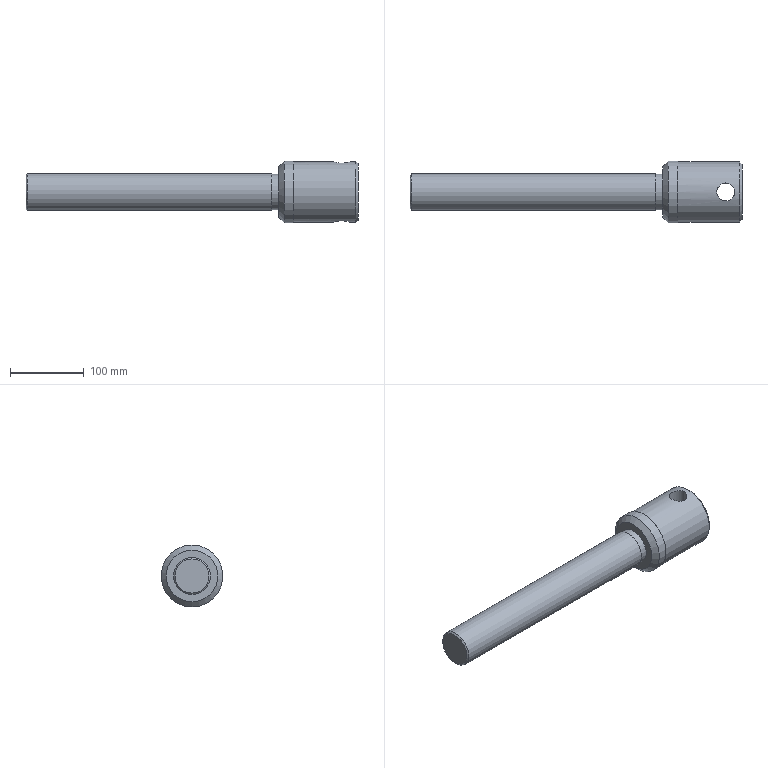Part | NX | features 侧推千斤顶活塞 2 | 1 solid | 13 faces | box 449.94 x 84 x 84 mm | volume 1201706 mm3 | plane 5 | cylinder 5 | cone 3 | commonest cylinder face diameters 24.29 x1 48 x1 50.16 x1 82 x1 84 x1
STEP:
#1=CARTESIAN_POINT('',(0.,0.,23.08));
#2=VERTEX_POINT('',#1);
#3=CARTESIAN_POINT('',(0.,0.,0.));
#4=DIRECTION('',(-1.,0.,0.));
#5=DIRECTION('',(0.,0.,1.));
#6=AXIS2_PLACEMENT_3D('',#3,#4,#5);
#7=CIRCLE('',#6,23.08);
#8=EDGE_CURVE('',#2,#2,#7,.T.);
#9=ORIENTED_EDGE('',*,*,#8,.T.);
#10=EDGE_LOOP('',(#9));
#11=FACE_BOUND('',#10,.T.);
#12=CARTESIAN_POINT('',(0.,0.,0.));
#13=DIRECTION('',(1.,0.,0.));
#14=DIRECTION('',(0.,0.,-1.));
#15=AXIS2_PLACEMENT_3D('',#12,#13,#14);
#16=PLANE('',#15);
#17=ADVANCED_FACE('',(#11),#16,.F.);
#18=ORIENTED_EDGE('',*,*,#8,.F.);
#19=EDGE_LOOP('',(#18));
#20=FACE_BOUND('',#19,.T.);
#21=CARTESIAN_POINT('',(2.,0.,25.08));
#22=VERTEX_POINT('',#21);
#23=CARTESIAN_POINT('',(2.,0.,0.));
#24=DIRECTION('',(-1.,0.,0.));
#25=DIRECTION('',(0.,0.,1.));
#26=AXIS2_PLACEMENT_3D('',#23,#24,#25);
#27=CIRCLE('',#26,25.08);
#28=EDGE_CURVE('',#22,#22,#27,.T.);
#29=ORIENTED_EDGE('',*,*,#28,.T.);
#30=EDGE_LOOP('',(#29));
#31=FACE_BOUND('',#30,.T.);
#32=CARTESIAN_POINT('',(2.,0.,0.));
#33=DIRECTION('',(1.,0.,0.));
#34=DIRECTION('',(0.,0.,-1.));
#35=AXIS2_PLACEMENT_3D('',#32,#33,#34);
#36=CONICAL_SURFACE('',#35,25.08,0.7854);
#37=ADVANCED_FACE('',(#20,#31),#36,.T.);
#38=ORIENTED_EDGE('',*,*,#28,.F.);
#39=EDGE_LOOP('',(#38));
#40=FACE_BOUND('',#39,.T.);
#41=CARTESIAN_POINT('',(332.85,0.,25.08));
#42=VERTEX_POINT('',#41);
#43=CARTESIAN_POINT('',(332.85,0.,0.));
#44=DIRECTION('',(-1.,0.,0.));
#45=DIRECTION('',(0.,0.,1.));
#46=AXIS2_PLACEMENT_3D('',#43,#44,#45);
#47=CIRCLE('',#46,25.08);
#48=EDGE_CURVE('',#42,#42,#47,.T.);
#49=ORIENTED_EDGE('',*,*,#48,.T.);
#50=EDGE_LOOP('',(#49));
#51=FACE_BOUND('',#50,.T.);
#52=CARTESIAN_POINT('',(0.,0.,0.));
#53=DIRECTION('',(-1.,0.,0.));
#54=DIRECTION('',(0.,0.,1.));
#55=AXIS2_PLACEMENT_3D('',#52,#53,#54);
#56=CYLINDRICAL_SURFACE('',#55,25.08);
#57=ADVANCED_FACE('',(#40,#51),#56,.T.);
#58=ORIENTED_EDGE('',*,*,#48,.F.);
#59=EDGE_LOOP('',(#58));
#60=FACE_BOUND('',#59,.T.);
#61=CARTESIAN_POINT('',(332.85,0.,24.));
#62=VERTEX_POINT('',#61);
#63=CARTESIAN_POINT('',(332.85,0.,0.));
#64=DIRECTION('',(-1.,0.,0.));
#65=DIRECTION('',(0.,0.,1.));
#66=AXIS2_PLACEMENT_3D('',#63,#64,#65);
#67=CIRCLE('',#66,24.);
#68=EDGE_CURVE('',#62,#62,#67,.T.);
#69=ORIENTED_EDGE('',*,*,#68,.T.);
#70=EDGE_LOOP('',(#69));
#71=FACE_BOUND('',#70,.T.);
#72=CARTESIAN_POINT('',(332.85,25.08,0.));
#73=DIRECTION('',(-1.,0.,0.));
#74=DIRECTION('',(0.,0.,1.));
#75=AXIS2_PLACEMENT_3D('',#72,#73,#74);
#76=PLANE('',#75);
#77=ADVANCED_FACE('',(#60,#71),#76,.F.);
#78=ORIENTED_EDGE('',*,*,#68,.F.);
#79=EDGE_LOOP('',(#78));
#80=FACE_BOUND('',#79,.T.);
#81=CARTESIAN_POINT('',(342.73,0.,24.));
#82=VERTEX_POINT('',#81);
#83=CARTESIAN_POINT('',(342.73,0.,0.));
#84=DIRECTION('',(-1.,0.,0.));
#85=DIRECTION('',(0.,0.,1.));
#86=AXIS2_PLACEMENT_3D('',#83,#84,#85);
#87=CIRCLE('',#86,24.);
#88=EDGE_CURVE('',#82,#82,#87,.T.);
#89=ORIENTED_EDGE('',*,*,#88,.T.);
#90=EDGE_LOOP('',(#89));
#91=FACE_BOUND('',#90,.T.);
#92=CARTESIAN_POINT('',(0.,0.,0.));
#93=DIRECTION('',(-1.,0.,0.));
#94=DIRECTION('',(0.,0.,1.));
#95=AXIS2_PLACEMENT_3D('',#92,#93,#94);
#96=CYLINDRICAL_SURFACE('',#95,24.);
#97=ADVANCED_FACE('',(#80,#91),#96,.T.);
#98=ORIENTED_EDGE('',*,*,#88,.F.);
#99=EDGE_LOOP('',(#98));
#100=FACE_BOUND('',#99,.T.);
#101=CARTESIAN_POINT('',(342.73,0.,34.86));
#102=VERTEX_POINT('',#101);
#103=CARTESIAN_POINT('',(342.73,0.,0.));
#104=DIRECTION('',(-1.,0.,0.));
#105=DIRECTION('',(0.,0.,1.));
#106=AXIS2_PLACEMENT_3D('',#103,#104,#105);
#107=CIRCLE('',#106,34.86);
#108=EDGE_CURVE('',#102,#102,#107,.T.);
#109=ORIENTED_EDGE('',*,*,#108,.T.);
#110=EDGE_LOOP('',(#109));
#111=FACE_BOUND('',#110,.T.);
#112=CARTESIAN_POINT('',(342.73,24.,0.));
#113=DIRECTION('',(1.,0.,0.));
#114=DIRECTION('',(0.,0.,-1.));
#115=AXIS2_PLACEMENT_3D('',#112,#113,#114);
#116=PLANE('',#115);
#117=ADVANCED_FACE('',(#100,#111),#116,.F.);
#118=ORIENTED_EDGE('',*,*,#108,.F.);
#119=EDGE_LOOP('',(#118));
#120=FACE_BOUND('',#119,.T.);
#121=CARTESIAN_POINT('',(349.87,0.,42.));
#122=VERTEX_POINT('',#121);
#123=CARTESIAN_POINT('',(349.87,0.,0.));
#124=DIRECTION('',(-1.,0.,0.));
#125=DIRECTION('',(0.,0.,1.));
#126=AXIS2_PLACEMENT_3D('',#123,#124,#125);
#127=CIRCLE('',#126,42.);
#128=EDGE_CURVE('',#122,#122,#127,.T.);
#129=ORIENTED_EDGE('',*,*,#128,.T.);
#130=EDGE_LOOP('',(#129));
#131=FACE_BOUND('',#130,.T.);
#132=CARTESIAN_POINT('',(349.87,0.,0.));
#133=DIRECTION('',(1.,0.,0.));
#134=DIRECTION('',(0.,0.,-1.));
#135=AXIS2_PLACEMENT_3D('',#132,#133,#134);
#136=CONICAL_SURFACE('',#135,42.,0.7854);
#137=ADVANCED_FACE('',(#120,#131),#136,.T.);
#138=ORIENTED_EDGE('',*,*,#128,.F.);
#139=EDGE_LOOP('',(#138));
#140=FACE_BOUND('',#139,.T.);
#141=CARTESIAN_POINT('',(362.94,0.,42.));
#142=VERTEX_POINT('',#141);
#143=CARTESIAN_POINT('',(362.94,0.,0.));
#144=DIRECTION('',(-1.,0.,0.));
#145=DIRECTION('',(0.,0.,1.));
#146=AXIS2_PLACEMENT_3D('',#143,#144,#145);
#147=CIRCLE('',#146,42.);
#148=EDGE_CURVE('',#142,#142,#147,.T.);
#149=ORIENTED_EDGE('',*,*,#148,.T.);
#150=EDGE_LOOP('',(#149));
#151=FACE_BOUND('',#150,.T.);
#152=CARTESIAN_POINT('',(0.,0.,0.));
#153=DIRECTION('',(-1.,0.,0.));
#154=DIRECTION('',(0.,0.,1.));
#155=AXIS2_PLACEMENT_3D('',#152,#153,#154);
#156=CYLINDRICAL_SURFACE('',#155,42.);
#157=ADVANCED_FACE('',(#140,#151),#156,.T.);
#158=ORIENTED_EDGE('',*,*,#148,.F.);
#159=EDGE_LOOP('',(#158));
#160=FACE_BOUND('',#159,.T.);
#161=CARTESIAN_POINT('',(362.94,0.,41.));
#162=VERTEX_POINT('',#161);
#163=CARTESIAN_POINT('',(362.94,0.,0.));
#164=DIRECTION('',(-1.,0.,0.));
#165=DIRECTION('',(0.,0.,1.));
#166=AXIS2_PLACEMENT_3D('',#163,#164,#165);
#167=CIRCLE('',#166,41.);
#168=EDGE_CURVE('',#162,#162,#167,.T.);
#169=ORIENTED_EDGE('',*,*,#168,.T.);
#170=EDGE_LOOP('',(#169));
#171=FACE_BOUND('',#170,.T.);
#172=CARTESIAN_POINT('',(362.94,42.,0.));
#173=DIRECTION('',(-1.,0.,0.));
#174=DIRECTION('',(0.,0.,1.));
#175=AXIS2_PLACEMENT_3D('',#172,#173,#174);
#176=PLANE('',#175);
#177=ADVANCED_FACE('',(#160,#171),#176,.F.);
#178=CARTESIAN_POINT('',(440.085,0.,41.));
#179=VERTEX_POINT('',#178);
#180=CARTESIAN_POINT('',(439.438,4.806,40.802));
#181=CARTESIAN_POINT('',(440.408,-0.002211,41.099));
#182=CARTESIAN_POINT('',(439.441,-4.797,40.802));
#183=CARTESIAN_POINT('',(436.744,-8.811,40.092));
#184=CARTESIAN_POINT('',(432.735,-11.5,39.368));
#185=CARTESIAN_POINT('',(427.95,-12.466,39.056));
#186=CARTESIAN_POINT('',(423.153,-11.506,39.366));
#187=CARTESIAN_POINT('',(419.13,-8.807,40.093));
#188=CARTESIAN_POINT('',(416.438,-4.793,40.803));
#189=CARTESIAN_POINT('',(415.474,-0.005926,41.098));
#190=CARTESIAN_POINT('',(416.434,4.785,40.804));
#191=CARTESIAN_POINT('',(419.128,8.804,40.094));
#192=CARTESIAN_POINT('',(423.143,11.501,39.368));
#193=CARTESIAN_POINT('',(427.936,12.466,39.056));
#194=CARTESIAN_POINT('',(432.729,11.504,39.367));
#195=CARTESIAN_POINT('',(436.743,8.811,40.092));
#196=CARTESIAN_POINT('',(439.438,4.806,40.802));
#197=CARTESIAN_POINT('',(440.408,-0.002211,41.099));
#198=CARTESIAN_POINT('',(439.441,-4.797,40.802));
#199=B_SPLINE_CURVE_WITH_KNOTS('',3,(#180,#181,#182,#183,#184,#185,#186,#187,#188,#189,#190,#191,#192,#193,#194,#195,#196,#197,#198),.UNSPECIFIED.,.T.,.F.,(1,1,1,1,1,1,1,1,1,1,1,1,1,1,1,1,1,1,1,1,1,1,1),(-0.01432,-0.009545,-0.004773,0.,0.004773,0.009545,0.01432,0.01909,0.02386,0.02864,0.03341,0.03818,0.04295,0.04773,0.0525,0.05727,0.06204,0.06682,0.07159,0.07636,0.08113,0.08591,0.09068),.UNSPECIFIED.);
#200=EDGE_CURVE('',#179,#179,#199,.T.);
#201=ORIENTED_EDGE('',*,*,#200,.T.);
#202=EDGE_LOOP('',(#201));
#203=FACE_BOUND('',#202,.T.);
#204=CARTESIAN_POINT('',(440.085,0.,-41.));
#205=VERTEX_POINT('',#204);
#206=CARTESIAN_POINT('',(439.438,-4.806,-40.802));
#207=CARTESIAN_POINT('',(440.408,0.002211,-41.099));
#208=CARTESIAN_POINT('',(439.441,4.797,-40.802));
#209=CARTESIAN_POINT('',(436.744,8.811,-40.092));
#210=CARTESIAN_POINT('',(432.735,11.5,-39.368));
#211=CARTESIAN_POINT('',(427.95,12.466,-39.056));
#212=CARTESIAN_POINT('',(423.153,11.506,-39.366));
#213=CARTESIAN_POINT('',(419.13,8.807,-40.093));
#214=CARTESIAN_POINT('',(416.438,4.793,-40.803));
#215=CARTESIAN_POINT('',(415.474,0.005926,-41.098));
#216=CARTESIAN_POINT('',(416.434,-4.785,-40.804));
#217=CARTESIAN_POINT('',(419.128,-8.804,-40.094));
#218=CARTESIAN_POINT('',(423.143,-11.501,-39.368));
#219=CARTESIAN_POINT('',(427.936,-12.466,-39.056));
#220=CARTESIAN_POINT('',(432.729,-11.504,-39.367));
#221=CARTESIAN_POINT('',(436.743,-8.811,-40.092));
#222=CARTESIAN_POINT('',(439.438,-4.806,-40.802));
#223=CARTESIAN_POINT('',(440.408,0.002211,-41.099));
#224=CARTESIAN_POINT('',(439.441,4.797,-40.802));
#225=B_SPLINE_CURVE_WITH_KNOTS('',3,(#206,#207,#208,#209,#210,#211,#212,#213,#214,#215,#216,#217,#218,#219,#220,#221,#222,#223,#224),.UNSPECIFIED.,.T.,.F.,(1,1,1,1,1,1,1,1,1,1,1,1,1,1,1,1,1,1,1,1,1,1,1),(-0.01432,-0.009545,-0.004773,0.,0.004773,0.009545,0.01432,0.01909,0.02386,0.02864,0.03341,0.03818,0.04295,0.04773,0.0525,0.05727,0.06204,0.06682,0.07159,0.07636,0.08113,0.08591,0.09068),.UNSPECIFIED.);
#226=EDGE_CURVE('',#205,#205,#225,.T.);
#227=ORIENTED_EDGE('',*,*,#226,.T.);
#228=EDGE_LOOP('',(#227));
#229=FACE_BOUND('',#228,.T.);
#230=ORIENTED_EDGE('',*,*,#168,.F.);
#231=EDGE_LOOP('',(#230));
#232=FACE_BOUND('',#231,.T.);
#233=CARTESIAN_POINT('',(446.94,0.,41.));
#234=VERTEX_POINT('',#233);
#235=CARTESIAN_POINT('',(446.94,0.,0.));
#236=DIRECTION('',(-1.,0.,0.));
#237=DIRECTION('',(0.,0.,1.));
#238=AXIS2_PLACEMENT_3D('',#235,#236,#237);
#239=CIRCLE('',#238,41.);
#240=EDGE_CURVE('',#234,#234,#239,.T.);
#241=ORIENTED_EDGE('',*,*,#240,.T.);
#242=EDGE_LOOP('',(#241));
#243=FACE_BOUND('',#242,.T.);
#244=CARTESIAN_POINT('',(0.,0.,0.));
#245=DIRECTION('',(-1.,0.,0.));
#246=DIRECTION('',(0.,0.,1.));
#247=AXIS2_PLACEMENT_3D('',#244,#245,#246);
#248=CYLINDRICAL_SURFACE('',#247,41.);
#249=ADVANCED_FACE('',(#203,#229,#232,#243),#248,.T.);
#250=ORIENTED_EDGE('',*,*,#240,.F.);
#251=EDGE_LOOP('',(#250));
#252=FACE_BOUND('',#251,.T.);
#253=CARTESIAN_POINT('',(449.94,0.,38.));
#254=VERTEX_POINT('',#253);
#255=CARTESIAN_POINT('',(449.94,0.,0.));
#256=DIRECTION('',(-1.,0.,0.));
#257=DIRECTION('',(0.,0.,1.));
#258=AXIS2_PLACEMENT_3D('',#255,#256,#257);
#259=CIRCLE('',#258,38.);
#260=EDGE_CURVE('',#254,#254,#259,.T.);
#261=ORIENTED_EDGE('',*,*,#260,.T.);
#262=EDGE_LOOP('',(#261));
#263=FACE_BOUND('',#262,.T.);
#264=CARTESIAN_POINT('',(449.94,0.,0.));
#265=DIRECTION('',(-1.,0.,0.));
#266=DIRECTION('',(0.,0.,1.));
#267=AXIS2_PLACEMENT_3D('',#264,#265,#266);
#268=CONICAL_SURFACE('',#267,38.,0.7854);
#269=ADVANCED_FACE('',(#252,#263),#268,.T.);
#270=ORIENTED_EDGE('',*,*,#260,.F.);
#271=EDGE_LOOP('',(#270));
#272=FACE_BOUND('',#271,.T.);
#273=CARTESIAN_POINT('',(449.94,38.,0.));
#274=DIRECTION('',(-1.,0.,0.));
#275=DIRECTION('',(0.,0.,1.));
#276=AXIS2_PLACEMENT_3D('',#273,#274,#275);
#277=PLANE('',#276);
#278=ADVANCED_FACE('',(#272),#277,.F.);
#279=ORIENTED_EDGE('',*,*,#226,.F.);
#280=EDGE_LOOP('',(#279));
#281=FACE_BOUND('',#280,.T.);
#282=ORIENTED_EDGE('',*,*,#200,.F.);
#283=EDGE_LOOP('',(#282));
#284=FACE_BOUND('',#283,.T.);
#285=CARTESIAN_POINT('',(427.94,0.,-53.5));
#286=DIRECTION('',(0.,0.,1.));
#287=DIRECTION('',(1.,0.,0.));
#288=AXIS2_PLACEMENT_3D('',#285,#286,#287);
#289=CYLINDRICAL_SURFACE('',#288,12.145);
#290=ADVANCED_FACE('',(#281,#284),#289,.F.);
#291=CLOSED_SHELL('',(#17,#37,#57,#77,#97,#117,#137,#157,#177,#249,#269,#278,#290));
#292=MANIFOLD_SOLID_BREP('',#291);
#293=(LENGTH_UNIT()NAMED_UNIT(*)SI_UNIT(.MILLI.,.METRE.));
#294=UNCERTAINTY_MEASURE_WITH_UNIT(LENGTH_MEASURE(0.0508),#293,'','');
#295=(NAMED_UNIT(*)PLANE_ANGLE_UNIT()SI_UNIT($,.RADIAN.));
#296=(NAMED_UNIT(*)SI_UNIT($,.STERADIAN.)SOLID_ANGLE_UNIT());
#297=(GEOMETRIC_REPRESENTATION_CONTEXT(3)GLOBAL_UNCERTAINTY_ASSIGNED_CONTEXT((#294))GLOBAL_UNIT_ASSIGNED_CONTEXT((#293,#295,#296))REPRESENTATION_CONTEXT('',''));
#298=ADVANCED_BREP_SHAPE_REPRESENTATION('',(#292),#297);